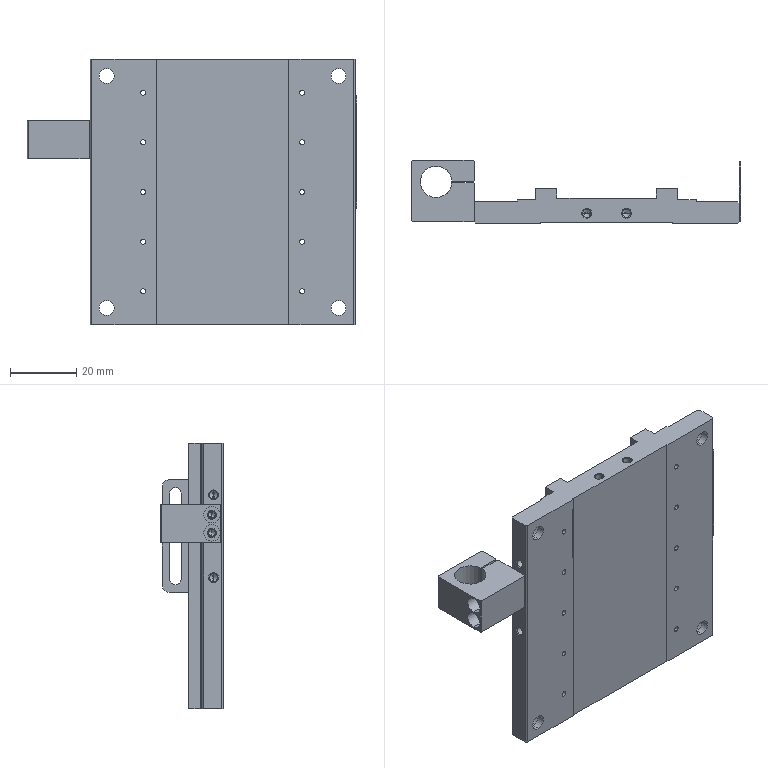Part | STEP file | E-EIC31-80-002 | 1 solid | 243 faces | box 99.5 x 19 x 80 mm | volume 49389 mm3 | cylinder 93 | cone 86 | plane 64 | commonest cylinder face diameters 2.459 x26 1.567 x20 2.013 x8 4.5 x8 8 x8 2.8 x4